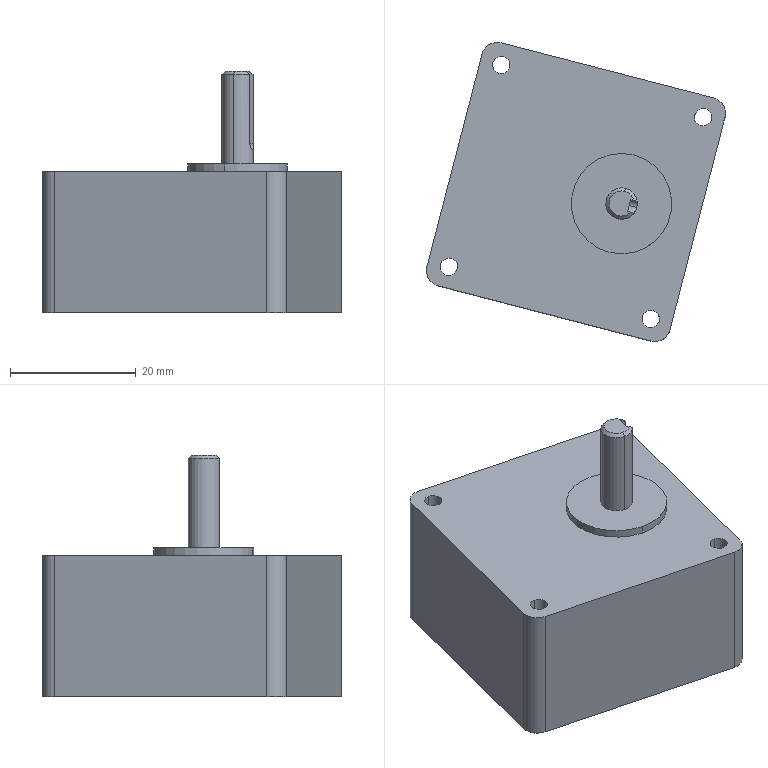Part | SolidWorks | features SplitBody 1 | 1 solid | 32 faces | box 47.65 x 47.65 x 38.5 mm | volume 35855 mm3 | cylinder 18 | plane 11 | cone 3 | commonest cylinder face diameters 2.75 x8 5 x6 2 x2 16 x2
STEP:
#1=CARTESIAN_POINT('',(-144.137,330.797,-440.116));
#2=VERTEX_POINT('',#1);
#3=CARTESIAN_POINT('',(-142.209,331.331,-440.116));
#4=VERTEX_POINT('',#3);
#5=CARTESIAN_POINT('',(-143.636,332.733,-440.116));
#6=DIRECTION('',(0.,0.,1.));
#7=DIRECTION('',(-0.2504,-0.9681,0.));
#8=AXIS2_PLACEMENT_3D('',#5,#6,#7);
#9=CIRCLE('',#8,2.);
#10=EDGE_CURVE('',#2,#4,#9,.T.);
#11=ORIENTED_EDGE('',*,*,#10,.F.);
#12=CARTESIAN_POINT('',(-144.262,330.313,-440.616));
#13=VERTEX_POINT('',#12);
#14=CARTESIAN_POINT('',(-144.137,330.797,-440.116));
#15=DIRECTION('',(-0.1771,-0.6846,-0.7071));
#16=VECTOR('',#15,1000.);
#17=LINE('',#14,#16);
#18=EDGE_CURVE('',#2,#13,#17,.T.);
#19=ORIENTED_EDGE('',*,*,#18,.T.);
#20=CARTESIAN_POINT('',(-141.668,331.191,-440.616));
#21=VERTEX_POINT('',#20);
#22=CARTESIAN_POINT('',(-143.636,332.733,-440.616));
#23=DIRECTION('',(0.,0.,-1.));
#24=DIRECTION('',(-0.2504,-0.9681,0.));
#25=AXIS2_PLACEMENT_3D('',#22,#23,#24);
#26=CIRCLE('',#25,2.5);
#27=EDGE_CURVE('',#21,#13,#26,.T.);
#28=ORIENTED_EDGE('',*,*,#27,.F.);
#29=CARTESIAN_POINT('',(-142.209,331.331,-440.116));
#30=CARTESIAN_POINT('',(-142.026,331.284,-440.279));
#31=CARTESIAN_POINT('',(-141.847,331.237,-440.447));
#32=CARTESIAN_POINT('',(-141.668,331.191,-440.616));
#33=B_SPLINE_CURVE_WITH_KNOTS('',3,(#29,#30,#31,#32),.UNSPECIFIED.,.F.,.F.,(4,4),(0.001662,0.002407),.UNSPECIFIED.);
#34=EDGE_CURVE('',#4,#21,#33,.T.);
#35=ORIENTED_EDGE('',*,*,#34,.F.);
#36=EDGE_LOOP('',(#11,#19,#28,#35));
#37=FACE_OUTER_BOUND('',#36,.T.);
#38=CARTESIAN_POINT('',(-143.636,332.733,-440.116));
#39=DIRECTION('',(0.,0.,-1.));
#40=DIRECTION('',(0.2504,0.9681,0.));
#41=AXIS2_PLACEMENT_3D('',#38,#39,#40);
#42=CONICAL_SURFACE('',#41,2.,0.7854);
#43=ADVANCED_FACE('',(#37),#42,.T.);
#44=ORIENTED_EDGE('',*,*,#18,.F.);
#45=CARTESIAN_POINT('',(-143.135,334.669,-440.116));
#46=VERTEX_POINT('',#45);
#47=CARTESIAN_POINT('',(-143.636,332.733,-440.116));
#48=DIRECTION('',(0.,0.,1.));
#49=DIRECTION('',(-0.2504,-0.9681,0.));
#50=AXIS2_PLACEMENT_3D('',#47,#48,#49);
#51=CIRCLE('',#50,2.);
#52=EDGE_CURVE('',#46,#2,#51,.T.);
#53=ORIENTED_EDGE('',*,*,#52,.F.);
#54=CARTESIAN_POINT('',(-143.01,335.153,-440.616));
#55=VERTEX_POINT('',#54);
#56=CARTESIAN_POINT('',(-143.135,334.669,-440.116));
#57=DIRECTION('',(0.1771,0.6846,-0.7071));
#58=VECTOR('',#57,1000.);
#59=LINE('',#56,#58);
#60=EDGE_CURVE('',#46,#55,#59,.T.);
#61=ORIENTED_EDGE('',*,*,#60,.T.);
#62=CARTESIAN_POINT('',(-143.636,332.733,-440.616));
#63=DIRECTION('',(0.,0.,-1.));
#64=DIRECTION('',(-0.2504,-0.9681,0.));
#65=AXIS2_PLACEMENT_3D('',#62,#63,#64);
#66=CIRCLE('',#65,2.5);
#67=EDGE_CURVE('',#13,#55,#66,.T.);
#68=ORIENTED_EDGE('',*,*,#67,.F.);
#69=EDGE_LOOP('',(#44,#53,#61,#68));
#70=FACE_OUTER_BOUND('',#69,.T.);
#71=CARTESIAN_POINT('',(-143.636,332.733,-440.116));
#72=DIRECTION('',(0.,0.,-1.));
#73=DIRECTION('',(0.2504,0.9681,0.));
#74=AXIS2_PLACEMENT_3D('',#71,#72,#73);
#75=CONICAL_SURFACE('',#74,2.,0.7854);
#76=ADVANCED_FACE('',(#70),#75,.T.);
#77=ORIENTED_EDGE('',*,*,#27,.T.);
#78=CARTESIAN_POINT('',(-144.262,330.313,-454.866));
#79=VERTEX_POINT('',#78);
#80=CARTESIAN_POINT('',(-144.262,330.313,-440.116));
#81=DIRECTION('',(0.,0.,-1.));
#82=VECTOR('',#81,1000.);
#83=LINE('',#80,#82);
#84=EDGE_CURVE('',#13,#79,#83,.T.);
#85=ORIENTED_EDGE('',*,*,#84,.T.);
#86=CARTESIAN_POINT('',(-143.01,335.153,-454.866));
#87=VERTEX_POINT('',#86);
#88=CARTESIAN_POINT('',(-143.636,332.733,-454.866));
#89=DIRECTION('',(0.,0.,-1.));
#90=DIRECTION('',(-0.2504,-0.9681,0.));
#91=AXIS2_PLACEMENT_3D('',#88,#89,#90);
#92=CIRCLE('',#91,2.5);
#93=EDGE_CURVE('',#87,#79,#92,.T.);
#94=ORIENTED_EDGE('',*,*,#93,.F.);
#95=CARTESIAN_POINT('',(-143.01,335.153,-440.116));
#96=DIRECTION('',(0.,0.,-1.));
#97=VECTOR('',#96,1000.);
#98=LINE('',#95,#97);
#99=EDGE_CURVE('',#55,#87,#98,.T.);
#100=ORIENTED_EDGE('',*,*,#99,.F.);
#101=CARTESIAN_POINT('',(-141.167,333.127,-440.616));
#102=VERTEX_POINT('',#101);
#103=CARTESIAN_POINT('',(-143.636,332.733,-440.616));
#104=DIRECTION('',(0.,0.,-1.));
#105=DIRECTION('',(-0.2504,-0.9681,0.));
#106=AXIS2_PLACEMENT_3D('',#103,#104,#105);
#107=CIRCLE('',#106,2.5);
#108=EDGE_CURVE('',#55,#102,#107,.T.);
#109=ORIENTED_EDGE('',*,*,#108,.T.);
#110=CARTESIAN_POINT('',(-141.167,333.127,-451.616));
#111=VERTEX_POINT('',#110);
#112=CARTESIAN_POINT('',(-141.167,333.127,-440.116));
#113=DIRECTION('',(0.,0.,-1.));
#114=VECTOR('',#113,1000.);
#115=LINE('',#112,#114);
#116=EDGE_CURVE('',#102,#111,#115,.T.);
#117=ORIENTED_EDGE('',*,*,#116,.T.);
#118=CARTESIAN_POINT('',(-141.216,332.107,-452.616));
#119=VERTEX_POINT('',#118);
#120=CARTESIAN_POINT('',(-141.167,333.127,-451.616));
#121=CARTESIAN_POINT('',(-141.167,333.127,-451.749));
#122=CARTESIAN_POINT('',(-141.162,333.098,-451.88));
#123=CARTESIAN_POINT('',(-141.149,332.991,-452.121));
#124=CARTESIAN_POINT('',(-141.141,332.912,-452.231));
#125=CARTESIAN_POINT('',(-141.134,332.722,-452.414));
#126=CARTESIAN_POINT('',(-141.136,332.609,-452.488));
#127=CARTESIAN_POINT('',(-141.16,332.367,-452.588));
#128=CARTESIAN_POINT('',(-141.182,332.236,-452.616));
#129=CARTESIAN_POINT('',(-141.216,332.107,-452.616));
#130=B_SPLINE_CURVE_WITH_KNOTS('',3,(#120,#121,#122,#123,#124,#125,#126,#127,#128,#129),.UNSPECIFIED.,.F.,.F.,(4,2,2,2,4),(0.,0.0003947,0.0007895,0.001184,0.001579),.UNSPECIFIED.);
#131=EDGE_CURVE('',#111,#119,#130,.T.);
#132=ORIENTED_EDGE('',*,*,#131,.T.);
#133=CARTESIAN_POINT('',(-141.668,331.191,-451.616));
#134=VERTEX_POINT('',#133);
#135=CARTESIAN_POINT('',(-141.216,332.107,-452.616));
#136=CARTESIAN_POINT('',(-141.249,331.978,-452.616));
#137=CARTESIAN_POINT('',(-141.292,331.854,-452.589));
#138=CARTESIAN_POINT('',(-141.389,331.629,-452.488));
#139=CARTESIAN_POINT('',(-141.443,331.529,-452.414));
#140=CARTESIAN_POINT('',(-141.54,331.366,-452.231));
#141=CARTESIAN_POINT('',(-141.586,331.301,-452.121));
#142=CARTESIAN_POINT('',(-141.649,331.214,-451.881));
#143=CARTESIAN_POINT('',(-141.668,331.191,-451.749));
#144=CARTESIAN_POINT('',(-141.668,331.191,-451.616));
#145=B_SPLINE_CURVE_WITH_KNOTS('',3,(#135,#136,#137,#138,#139,#140,#141,#142,#143,#144),.UNSPECIFIED.,.F.,.F.,(4,2,2,2,4),(0.,0.0003948,0.0007895,0.001184,0.001579),.UNSPECIFIED.);
#146=EDGE_CURVE('',#119,#134,#145,.T.);
#147=ORIENTED_EDGE('',*,*,#146,.T.);
#148=CARTESIAN_POINT('',(-141.668,331.191,-440.116));
#149=DIRECTION('',(0.,0.,1.));
#150=VECTOR('',#149,1000.);
#151=LINE('',#148,#150);
#152=EDGE_CURVE('',#134,#21,#151,.T.);
#153=ORIENTED_EDGE('',*,*,#152,.T.);
#154=EDGE_LOOP('',(#77,#85,#94,#100,#109,#117,#132,#147,#153));
#155=FACE_OUTER_BOUND('',#154,.T.);
#156=CARTESIAN_POINT('',(-143.636,332.733,-440.116));
#157=DIRECTION('',(0.,0.,-1.));
#158=DIRECTION('',(0.2504,0.9681,0.));
#159=AXIS2_PLACEMENT_3D('',#156,#157,#158);
#160=CYLINDRICAL_SURFACE('',#159,2.5);
#161=ADVANCED_FACE('',(#155),#160,.T.);
#162=CARTESIAN_POINT('',(-145.639,324.988,-454.866));
#163=VERTEX_POINT('',#162);
#164=CARTESIAN_POINT('',(-141.632,340.478,-454.866));
#165=VERTEX_POINT('',#164);
#166=CARTESIAN_POINT('',(-143.636,332.733,-454.866));
#167=DIRECTION('',(0.,0.,1.));
#168=DIRECTION('',(-0.2504,-0.9681,0.));
#169=AXIS2_PLACEMENT_3D('',#166,#167,#168);
#170=CIRCLE('',#169,8.);
#171=EDGE_CURVE('',#163,#165,#170,.T.);
#172=ORIENTED_EDGE('',*,*,#171,.F.);
#173=CARTESIAN_POINT('',(-145.639,324.988,-456.116));
#174=VERTEX_POINT('',#173);
#175=CARTESIAN_POINT('',(-145.639,324.988,-454.866));
#176=DIRECTION('',(0.,0.,-1.));
#177=VECTOR('',#176,1000.);
#178=LINE('',#175,#177);
#179=EDGE_CURVE('',#163,#174,#178,.T.);
#180=ORIENTED_EDGE('',*,*,#179,.T.);
#181=CARTESIAN_POINT('',(-141.632,340.478,-456.116));
#182=VERTEX_POINT('',#181);
#183=CARTESIAN_POINT('',(-143.636,332.733,-456.116));
#184=DIRECTION('',(0.,0.,1.));
#185=DIRECTION('',(-0.2504,-0.9681,0.));
#186=AXIS2_PLACEMENT_3D('',#183,#184,#185);
#187=CIRCLE('',#186,8.);
#188=EDGE_CURVE('',#174,#182,#187,.T.);
#189=ORIENTED_EDGE('',*,*,#188,.T.);
#190=CARTESIAN_POINT('',(-141.632,340.478,-454.866));
#191=DIRECTION('',(0.,0.,-1.));
#192=VECTOR('',#191,1000.);
#193=LINE('',#190,#192);
#194=EDGE_CURVE('',#165,#182,#193,.T.);
#195=ORIENTED_EDGE('',*,*,#194,.F.);
#196=EDGE_LOOP('',(#172,#180,#189,#195));
#197=FACE_OUTER_BOUND('',#196,.T.);
#198=CARTESIAN_POINT('',(-143.636,332.733,-454.866));
#199=DIRECTION('',(0.,0.,-1.));
#200=DIRECTION('',(0.2504,0.9681,0.));
#201=AXIS2_PLACEMENT_3D('',#198,#199,#200);
#202=CYLINDRICAL_SURFACE('',#201,8.);
#203=ADVANCED_FACE('',(#197),#202,.T.);
#204=CARTESIAN_POINT('',(-138.627,315.693,-456.116));
#205=VERTEX_POINT('',#204);
#206=CARTESIAN_POINT('',(-139.315,313.031,-456.116));
#207=VERTEX_POINT('',#206);
#208=CARTESIAN_POINT('',(-138.971,314.362,-456.116));
#209=DIRECTION('',(0.,0.,1.));
#210=DIRECTION('',(-0.2504,-0.9681,0.));
#211=AXIS2_PLACEMENT_3D('',#208,#209,#210);
#212=CIRCLE('',#211,1.375);
#213=EDGE_CURVE('',#205,#207,#212,.T.);
#214=ORIENTED_EDGE('',*,*,#213,.T.);
#215=CARTESIAN_POINT('',(-139.315,313.031,-478.616));
#216=VERTEX_POINT('',#215);
#217=CARTESIAN_POINT('',(-139.315,313.031,-456.116));
#218=DIRECTION('',(0.,0.,-1.));
#219=VECTOR('',#218,1000.);
#220=LINE('',#217,#219);
#221=EDGE_CURVE('',#207,#216,#220,.T.);
#222=ORIENTED_EDGE('',*,*,#221,.T.);
#223=CARTESIAN_POINT('',(-138.627,315.693,-478.616));
#224=VERTEX_POINT('',#223);
#225=CARTESIAN_POINT('',(-138.971,314.362,-478.616));
#226=DIRECTION('',(0.,0.,1.));
#227=DIRECTION('',(-0.2504,-0.9681,0.));
#228=AXIS2_PLACEMENT_3D('',#225,#226,#227);
#229=CIRCLE('',#228,1.375);
#230=EDGE_CURVE('',#224,#216,#229,.T.);
#231=ORIENTED_EDGE('',*,*,#230,.F.);
#232=CARTESIAN_POINT('',(-138.627,315.693,-456.116));
#233=DIRECTION('',(0.,0.,-1.));
#234=VECTOR('',#233,1000.);
#235=LINE('',#232,#234);
#236=EDGE_CURVE('',#205,#224,#235,.T.);
#237=ORIENTED_EDGE('',*,*,#236,.F.);
#238=EDGE_LOOP('',(#214,#222,#231,#237));
#239=FACE_OUTER_BOUND('',#238,.T.);
#240=CARTESIAN_POINT('',(-138.971,314.362,-456.116));
#241=DIRECTION('',(0.,0.,-1.));
#242=DIRECTION('',(0.2504,0.9681,0.));
#243=AXIS2_PLACEMENT_3D('',#240,#241,#242);
#244=CYLINDRICAL_SURFACE('',#243,1.375);
#245=ADVANCED_FACE('',(#239),#244,.F.);
#246=CARTESIAN_POINT('',(-170.802,324.017,-456.116));
#247=VERTEX_POINT('',#246);
#248=CARTESIAN_POINT('',(-171.49,321.354,-456.116));
#249=VERTEX_POINT('',#248);
#250=CARTESIAN_POINT('',(-171.146,322.685,-456.116));
#251=DIRECTION('',(0.,0.,1.));
#252=DIRECTION('',(-0.2504,-0.9681,0.));
#253=AXIS2_PLACEMENT_3D('',#250,#251,#252);
#254=CIRCLE('',#253,1.375);
#255=EDGE_CURVE('',#247,#249,#254,.T.);
#256=ORIENTED_EDGE('',*,*,#255,.T.);
#257=CARTESIAN_POINT('',(-171.49,321.354,-478.616));
#258=VERTEX_POINT('',#257);
#259=CARTESIAN_POINT('',(-171.49,321.354,-456.116));
#260=DIRECTION('',(0.,0.,-1.));
#261=VECTOR('',#260,1000.);
#262=LINE('',#259,#261);
#263=EDGE_CURVE('',#249,#258,#262,.T.);
#264=ORIENTED_EDGE('',*,*,#263,.T.);
#265=CARTESIAN_POINT('',(-170.802,324.017,-478.616));
#266=VERTEX_POINT('',#265);
#267=CARTESIAN_POINT('',(-171.146,322.685,-478.616));
#268=DIRECTION('',(0.,0.,1.));
#269=DIRECTION('',(-0.2504,-0.9681,0.));
#270=AXIS2_PLACEMENT_3D('',#267,#268,#269);
#271=CIRCLE('',#270,1.375);
#272=EDGE_CURVE('',#266,#258,#271,.T.);
#273=ORIENTED_EDGE('',*,*,#272,.F.);
#274=CARTESIAN_POINT('',(-170.802,324.017,-456.116));
#275=DIRECTION('',(0.,0.,-1.));
#276=VECTOR('',#275,1000.);
#277=LINE('',#274,#276);
#278=EDGE_CURVE('',#247,#266,#277,.T.);
#279=ORIENTED_EDGE('',*,*,#278,.F.);
#280=EDGE_LOOP('',(#256,#264,#273,#279));
#281=FACE_OUTER_BOUND('',#280,.T.);
#282=CARTESIAN_POINT('',(-171.146,322.685,-456.116));
#283=DIRECTION('',(0.,0.,-1.));
#284=DIRECTION('',(0.2504,0.9681,0.));
#285=AXIS2_PLACEMENT_3D('',#282,#283,#284);
#286=CYLINDRICAL_SURFACE('',#285,1.375);
#287=ADVANCED_FACE('',(#281),#286,.F.);
#288=CARTESIAN_POINT('',(-162.478,356.191,-456.116));
#289=VERTEX_POINT('',#288);
#290=CARTESIAN_POINT('',(-163.167,353.529,-456.116));
#291=VERTEX_POINT('',#290);
#292=CARTESIAN_POINT('',(-162.823,354.86,-456.116));
#293=DIRECTION('',(0.,0.,1.));
#294=DIRECTION('',(-0.2504,-0.9681,0.));
#295=AXIS2_PLACEMENT_3D('',#292,#293,#294);
#296=CIRCLE('',#295,1.375);
#297=EDGE_CURVE('',#289,#291,#296,.T.);
#298=ORIENTED_EDGE('',*,*,#297,.T.);
#299=CARTESIAN_POINT('',(-163.167,353.529,-478.616));
#300=VERTEX_POINT('',#299);
#301=CARTESIAN_POINT('',(-163.167,353.529,-456.116));
#302=DIRECTION('',(0.,0.,-1.));
#303=VECTOR('',#302,1000.);
#304=LINE('',#301,#303);
#305=EDGE_CURVE('',#291,#300,#304,.T.);
#306=ORIENTED_EDGE('',*,*,#305,.T.);
#307=CARTESIAN_POINT('',(-162.478,356.191,-478.616));
#308=VERTEX_POINT('',#307);
#309=CARTESIAN_POINT('',(-162.823,354.86,-478.616));
#310=DIRECTION('',(0.,0.,1.));
#311=DIRECTION('',(-0.2504,-0.9681,0.));
#312=AXIS2_PLACEMENT_3D('',#309,#310,#311);
#313=CIRCLE('',#312,1.375);
#314=EDGE_CURVE('',#308,#300,#313,.T.);
#315=ORIENTED_EDGE('',*,*,#314,.F.);
#316=CARTESIAN_POINT('',(-162.478,356.191,-456.116));
#317=DIRECTION('',(0.,0.,-1.));
#318=VECTOR('',#317,1000.);
#319=LINE('',#316,#318);
#320=EDGE_CURVE('',#289,#308,#319,.T.);
#321=ORIENTED_EDGE('',*,*,#320,.F.);
#322=EDGE_LOOP('',(#298,#306,#315,#321));
#323=FACE_OUTER_BOUND('',#322,.T.);
#324=CARTESIAN_POINT('',(-162.823,354.86,-456.116));
#325=DIRECTION('',(0.,0.,-1.));
#326=DIRECTION('',(0.2504,0.9681,0.));
#327=AXIS2_PLACEMENT_3D('',#324,#325,#326);
#328=CYLINDRICAL_SURFACE('',#327,1.375);
#329=ADVANCED_FACE('',(#323),#328,.F.);
#330=CARTESIAN_POINT('',(-130.304,347.868,-456.116));
#331=VERTEX_POINT('',#330);
#332=CARTESIAN_POINT('',(-130.992,345.206,-456.116));
#333=VERTEX_POINT('',#332);
#334=CARTESIAN_POINT('',(-130.648,346.537,-456.116));
#335=DIRECTION('',(0.,0.,1.));
#336=DIRECTION('',(-0.2504,-0.9681,0.));
#337=AXIS2_PLACEMENT_3D('',#334,#335,#336);
#338=CIRCLE('',#337,1.375);
#339=EDGE_CURVE('',#331,#333,#338,.T.);
#340=ORIENTED_EDGE('',*,*,#339,.T.);
#341=CARTESIAN_POINT('',(-130.992,345.206,-478.616));
#342=VERTEX_POINT('',#341);
#343=CARTESIAN_POINT('',(-130.992,345.206,-456.116));
#344=DIRECTION('',(0.,0.,-1.));
#345=VECTOR('',#344,1000.);
#346=LINE('',#343,#345);
#347=EDGE_CURVE('',#333,#342,#346,.T.);
#348=ORIENTED_EDGE('',*,*,#347,.T.);
#349=CARTESIAN_POINT('',(-130.304,347.868,-478.616));
#350=VERTEX_POINT('',#349);
#351=CARTESIAN_POINT('',(-130.648,346.537,-478.616));
#352=DIRECTION('',(0.,0.,1.));
#353=DIRECTION('',(-0.2504,-0.9681,0.));
#354=AXIS2_PLACEMENT_3D('',#351,#352,#353);
#355=CIRCLE('',#354,1.375);
#356=EDGE_CURVE('',#350,#342,#355,.T.);
#357=ORIENTED_EDGE('',*,*,#356,.F.);
#358=CARTESIAN_POINT('',(-130.304,347.868,-456.116));
#359=DIRECTION('',(0.,0.,-1.));
#360=VECTOR('',#359,1000.);
#361=LINE('',#358,#360);
#362=EDGE_CURVE('',#331,#350,#361,.T.);
#363=ORIENTED_EDGE('',*,*,#362,.F.);
#364=EDGE_LOOP('',(#340,#348,#357,#363));
#365=FACE_OUTER_BOUND('',#364,.T.);
#366=CARTESIAN_POINT('',(-130.648,346.537,-456.116));
#367=DIRECTION('',(0.,0.,-1.));
#368=DIRECTION('',(0.2504,0.9681,0.));
#369=AXIS2_PLACEMENT_3D('',#366,#367,#368);
#370=CYLINDRICAL_SURFACE('',#369,1.375);
#371=ADVANCED_FACE('',(#365),#370,.F.);
#372=CARTESIAN_POINT('',(-143.636,332.733,-454.866));
#373=DIRECTION('',(0.,0.,1.));
#374=DIRECTION('',(-0.2504,-0.9681,0.));
#375=AXIS2_PLACEMENT_3D('',#372,#373,#374);
#376=CIRCLE('',#375,8.);
#377=EDGE_CURVE('',#165,#163,#376,.T.);
#378=ORIENTED_EDGE('',*,*,#377,.T.);
#379=ORIENTED_EDGE('',*,*,#171,.T.);
#380=EDGE_LOOP('',(#378,#379));
#381=FACE_OUTER_BOUND('',#380,.T.);
#382=ORIENTED_EDGE('',*,*,#93,.T.);
#383=CARTESIAN_POINT('',(-143.636,332.733,-454.866));
#384=DIRECTION('',(0.,0.,-1.));
#385=DIRECTION('',(-0.2504,-0.9681,0.));
#386=AXIS2_PLACEMENT_3D('',#383,#384,#385);
#387=CIRCLE('',#386,2.5);
#388=EDGE_CURVE('',#79,#87,#387,.T.);
#389=ORIENTED_EDGE('',*,*,#388,.T.);
#390=EDGE_LOOP('',(#382,#389));
#391=FACE_BOUND('',#390,.T.);
#392=CARTESIAN_POINT('',(-143.636,332.733,-454.866));
#393=DIRECTION('',(0.,0.,1.));
#394=DIRECTION('',(-0.2504,-0.9681,0.));
#395=AXIS2_PLACEMENT_3D('',#392,#393,#394);
#396=PLANE('',#395);
#397=ADVANCED_FACE('',(#381,#391),#396,.T.);
#398=ORIENTED_EDGE('',*,*,#213,.F.);
#399=CARTESIAN_POINT('',(-138.971,314.362,-456.116));
#400=DIRECTION('',(0.,0.,1.));
#401=DIRECTION('',(-0.2504,-0.9681,0.));
#402=AXIS2_PLACEMENT_3D('',#399,#400,#401);
#403=CIRCLE('',#402,1.375);
#404=EDGE_CURVE('',#207,#205,#403,.T.);
#405=ORIENTED_EDGE('',*,*,#404,.F.);
#406=EDGE_LOOP('',(#398,#405));
#407=FACE_BOUND('',#406,.T.);
#408=ORIENTED_EDGE('',*,*,#297,.F.);
#409=CARTESIAN_POINT('',(-162.823,354.86,-456.116));
#410=DIRECTION('',(0.,0.,1.));
#411=DIRECTION('',(-0.2504,-0.9681,0.));
#412=AXIS2_PLACEMENT_3D('',#409,#410,#411);
#413=CIRCLE('',#412,1.375);
#414=EDGE_CURVE('',#291,#289,#413,.T.);
#415=ORIENTED_EDGE('',*,*,#414,.F.);
#416=EDGE_LOOP('',(#408,#415));
#417=FACE_BOUND('',#416,.T.);
#418=CARTESIAN_POINT('',(-162.83,358.357,-456.116));
#419=VERTEX_POINT('',#418);
#420=CARTESIAN_POINT('',(-165.877,356.562,-456.116));
#421=VERTEX_POINT('',#420);
#422=CARTESIAN_POINT('',(-163.457,355.936,-456.116));
#423=DIRECTION('',(0.,0.,1.));
#424=DIRECTION('',(-0.2504,-0.9681,0.));
#425=AXIS2_PLACEMENT_3D('',#422,#423,#424);
#426=CIRCLE('',#425,2.5);
#427=EDGE_CURVE('',#419,#421,#426,.T.);
#428=ORIENTED_EDGE('',*,*,#427,.T.);
#429=CARTESIAN_POINT('',(-174.642,322.678,-456.116));
#430=VERTEX_POINT('',#429);
#431=CARTESIAN_POINT('',(-165.877,356.562,-456.116));
#432=DIRECTION('',(-0.2504,-0.9681,0.));
#433=VECTOR('',#432,1000.);
#434=LINE('',#431,#433);
#435=EDGE_CURVE('',#421,#430,#434,.T.);
#436=ORIENTED_EDGE('',*,*,#435,.T.);
#437=CARTESIAN_POINT('',(-172.848,319.631,-456.116));
#438=VERTEX_POINT('',#437);
#439=CARTESIAN_POINT('',(-172.222,322.052,-456.116));
#440=DIRECTION('',(0.,0.,1.));
#441=DIRECTION('',(-0.2504,-0.9681,0.));
#442=AXIS2_PLACEMENT_3D('',#439,#440,#441);
#443=CIRCLE('',#442,2.5);
#444=EDGE_CURVE('',#430,#438,#443,.T.);
#445=ORIENTED_EDGE('',*,*,#444,.T.);
#446=CARTESIAN_POINT('',(-138.963,310.866,-456.116));
#447=VERTEX_POINT('',#446);
#448=CARTESIAN_POINT('',(-172.848,319.631,-456.116));
#449=DIRECTION('',(0.9681,-0.2504,0.));
#450=VECTOR('',#449,1000.);
#451=LINE('',#448,#450);
#452=EDGE_CURVE('',#438,#447,#451,.T.);
#453=ORIENTED_EDGE('',*,*,#452,.T.);
#454=CARTESIAN_POINT('',(-135.917,312.66,-456.116));
#455=VERTEX_POINT('',#454);
#456=CARTESIAN_POINT('',(-138.337,313.286,-456.116));
#457=DIRECTION('',(0.,0.,1.));
#458=DIRECTION('',(-0.2504,-0.9681,0.));
#459=AXIS2_PLACEMENT_3D('',#456,#457,#458);
#460=CIRCLE('',#459,2.5);
#461=EDGE_CURVE('',#447,#455,#460,.T.);
#462=ORIENTED_EDGE('',*,*,#461,.T.);
#463=CARTESIAN_POINT('',(-127.152,346.545,-456.116));
#464=VERTEX_POINT('',#463);
#465=CARTESIAN_POINT('',(-135.917,312.66,-456.116));
#466=DIRECTION('',(0.2504,0.9681,0.));
#467=VECTOR('',#466,1000.);
#468=LINE('',#465,#467);
#469=EDGE_CURVE('',#455,#464,#468,.T.);
#470=ORIENTED_EDGE('',*,*,#469,.T.);
#471=CARTESIAN_POINT('',(-128.946,349.591,-456.116));
#472=VERTEX_POINT('',#471);
#473=CARTESIAN_POINT('',(-129.572,347.171,-456.116));
#474=DIRECTION('',(0.,0.,1.));
#475=DIRECTION('',(-0.2504,-0.9681,0.));
#476=AXIS2_PLACEMENT_3D('',#473,#474,#475);
#477=CIRCLE('',#476,2.5);
#478=EDGE_CURVE('',#464,#472,#477,.T.);
#479=ORIENTED_EDGE('',*,*,#478,.T.);
#480=CARTESIAN_POINT('',(-128.946,349.591,-456.116));
#481=DIRECTION('',(-0.9681,0.2504,0.));
#482=VECTOR('',#481,1000.);
#483=LINE('',#480,#482);
#484=EDGE_CURVE('',#472,#419,#483,.T.);
#485=ORIENTED_EDGE('',*,*,#484,.T.);
#486=EDGE_LOOP('',(#428,#436,#445,#453,#462,#470,#479,#485));
#487=FACE_OUTER_BOUND('',#486,.T.);
#488=ORIENTED_EDGE('',*,*,#339,.F.);
#489=CARTESIAN_POINT('',(-130.648,346.537,-456.116));
#490=DIRECTION('',(0.,0.,1.));
#491=DIRECTION('',(-0.2504,-0.9681,0.));
#492=AXIS2_PLACEMENT_3D('',#489,#490,#491);
#493=CIRCLE('',#492,1.375);
#494=EDGE_CURVE('',#333,#331,#493,.T.);
#495=ORIENTED_EDGE('',*,*,#494,.F.);
#496=EDGE_LOOP('',(#488,#495));
#497=FACE_BOUND('',#496,.T.);
#498=ORIENTED_EDGE('',*,*,#255,.F.);
#499=CARTESIAN_POINT('',(-171.146,322.685,-456.116));
#500=DIRECTION('',(0.,0.,1.));
#501=DIRECTION('',(-0.2504,-0.9681,0.));
#502=AXIS2_PLACEMENT_3D('',#499,#500,#501);
#503=CIRCLE('',#502,1.375);
#504=EDGE_CURVE('',#249,#247,#503,.T.);
#505=ORIENTED_EDGE('',*,*,#504,.F.);
#506=EDGE_LOOP('',(#498,#505));
#507=FACE_BOUND('',#506,.T.);
#508=CARTESIAN_POINT('',(-143.636,332.733,-456.116));
#509=DIRECTION('',(0.,0.,1.));
#510=DIRECTION('',(-0.2504,-0.9681,0.));
#511=AXIS2_PLACEMENT_3D('',#508,#509,#510);
#512=CIRCLE('',#511,8.);
#513=EDGE_CURVE('',#182,#174,#512,.T.);
#514=ORIENTED_EDGE('',*,*,#513,.F.);
#515=ORIENTED_EDGE('',*,*,#188,.F.);
#516=EDGE_LOOP('',(#514,#515));
#517=FACE_BOUND('',#516,.T.);
#518=CARTESIAN_POINT('',(-163.457,355.936,-456.116));
#519=DIRECTION('',(0.,0.,1.));
#520=DIRECTION('',(-0.2504,-0.9681,0.));
#521=AXIS2_PLACEMENT_3D('',#518,#519,#520);
#522=PLANE('',#521);
#523=ADVANCED_FACE('',(#407,#417,#487,#497,#507,#517),#522,.T.);
#524=ORIENTED_EDGE('',*,*,#272,.T.);
#525=CARTESIAN_POINT('',(-171.146,322.685,-478.616));
#526=DIRECTION('',(0.,0.,1.));
#527=DIRECTION('',(-0.2504,-0.9681,0.));
#528=AXIS2_PLACEMENT_3D('',#525,#526,#527);
#529=CIRCLE('',#528,1.375);
#530=EDGE_CURVE('',#258,#266,#529,.T.);
#531=ORIENTED_EDGE('',*,*,#530,.T.);
#532=EDGE_LOOP('',(#524,#531));
#533=FACE_BOUND('',#532,.T.);
#534=ORIENTED_EDGE('',*,*,#356,.T.);
#535=CARTESIAN_POINT('',(-130.648,346.537,-478.616));
#536=DIRECTION('',(0.,0.,1.));
#537=DIRECTION('',(-0.2504,-0.9681,0.));
#538=AXIS2_PLACEMENT_3D('',#535,#536,#537);
#539=CIRCLE('',#538,1.375);
#540=EDGE_CURVE('',#342,#350,#539,.T.);
#541=ORIENTED_EDGE('',*,*,#540,.T.);
#542=EDGE_LOOP('',(#534,#541));
#543=FACE_BOUND('',#542,.T.);
#544=CARTESIAN_POINT('',(-162.83,358.357,-478.616));
#545=VERTEX_POINT('',#544);
#546=CARTESIAN_POINT('',(-165.877,356.562,-478.616));
#547=VERTEX_POINT('',#546);
#548=CARTESIAN_POINT('',(-163.457,355.936,-478.616));
#549=DIRECTION('',(0.,0.,1.));
#550=DIRECTION('',(-0.2504,-0.9681,0.));
#551=AXIS2_PLACEMENT_3D('',#548,#549,#550);
#552=CIRCLE('',#551,2.5);
#553=EDGE_CURVE('',#545,#547,#552,.T.);
#554=ORIENTED_EDGE('',*,*,#553,.F.);
#555=CARTESIAN_POINT('',(-128.946,349.591,-478.616));
#556=VERTEX_POINT('',#555);
#557=CARTESIAN_POINT('',(-128.946,349.591,-478.616));
#558=DIRECTION('',(-0.9681,0.2504,0.));
#559=VECTOR('',#558,1000.);
#560=LINE('',#557,#559);
#561=EDGE_CURVE('',#556,#545,#560,.T.);
#562=ORIENTED_EDGE('',*,*,#561,.F.);
#563=CARTESIAN_POINT('',(-127.152,346.545,-478.616));
#564=VERTEX_POINT('',#563);
#565=CARTESIAN_POINT('',(-129.572,347.171,-478.616));
#566=DIRECTION('',(0.,0.,1.));
#567=DIRECTION('',(-0.2504,-0.9681,0.));
#568=AXIS2_PLACEMENT_3D('',#565,#566,#567);
#569=CIRCLE('',#568,2.5);
#570=EDGE_CURVE('',#564,#556,#569,.T.);
#571=ORIENTED_EDGE('',*,*,#570,.F.);
#572=CARTESIAN_POINT('',(-135.917,312.66,-478.616));
#573=VERTEX_POINT('',#572);
#574=CARTESIAN_POINT('',(-135.917,312.66,-478.616));
#575=DIRECTION('',(0.2504,0.9681,0.));
#576=VECTOR('',#575,1000.);
#577=LINE('',#574,#576);
#578=EDGE_CURVE('',#573,#564,#577,.T.);
#579=ORIENTED_EDGE('',*,*,#578,.F.);
#580=CARTESIAN_POINT('',(-138.963,310.866,-478.616));
#581=VERTEX_POINT('',#580);
#582=CARTESIAN_POINT('',(-138.337,313.286,-478.616));
#583=DIRECTION('',(0.,0.,1.));
#584=DIRECTION('',(-0.2504,-0.9681,0.));
#585=AXIS2_PLACEMENT_3D('',#582,#583,#584);
#586=CIRCLE('',#585,2.5);
#587=EDGE_CURVE('',#581,#573,#586,.T.);
#588=ORIENTED_EDGE('',*,*,#587,.F.);
#589=CARTESIAN_POINT('',(-172.848,319.631,-478.616));
#590=VERTEX_POINT('',#589);
#591=CARTESIAN_POINT('',(-172.848,319.631,-478.616));
#592=DIRECTION('',(0.9681,-0.2504,0.));
#593=VECTOR('',#592,1000.);
#594=LINE('',#591,#593);
#595=EDGE_CURVE('',#590,#581,#594,.T.);
#596=ORIENTED_EDGE('',*,*,#595,.F.);
#597=CARTESIAN_POINT('',(-174.642,322.678,-478.616));
#598=VERTEX_POINT('',#597);
#599=CARTESIAN_POINT('',(-172.222,322.052,-478.616));
#600=DIRECTION('',(0.,0.,1.));
#601=DIRECTION('',(-0.2504,-0.9681,0.));
#602=AXIS2_PLACEMENT_3D('',#599,#600,#601);
#603=CIRCLE('',#602,2.5);
#604=EDGE_CURVE('',#598,#590,#603,.T.);
#605=ORIENTED_EDGE('',*,*,#604,.F.);
#606=CARTESIAN_POINT('',(-165.877,356.562,-478.616));
#607=DIRECTION('',(-0.2504,-0.9681,0.));
#608=VECTOR('',#607,1000.);
#609=LINE('',#606,#608);
#610=EDGE_CURVE('',#547,#598,#609,.T.);
#611=ORIENTED_EDGE('',*,*,#610,.F.);
#612=EDGE_LOOP('',(#554,#562,#571,#579,#588,#596,#605,#611));
#613=FACE_OUTER_BOUND('',#612,.T.);
#614=ORIENTED_EDGE('',*,*,#314,.T.);
#615=CARTESIAN_POINT('',(-162.823,354.86,-478.616));
#616=DIRECTION('',(0.,0.,1.));
#617=DIRECTION('',(-0.2504,-0.9681,0.));
#618=AXIS2_PLACEMENT_3D('',#615,#616,#617);
#619=CIRCLE('',#618,1.375);
#620=EDGE_CURVE('',#300,#308,#619,.T.);
#621=ORIENTED_EDGE('',*,*,#620,.T.);
#622=EDGE_LOOP('',(#614,#621));
#623=FACE_BOUND('',#622,.T.);
#624=ORIENTED_EDGE('',*,*,#230,.T.);
#625=CARTESIAN_POINT('',(-138.971,314.362,-478.616));
#626=DIRECTION('',(0.,0.,1.));
#627=DIRECTION('',(-0.2504,-0.9681,0.));
#628=AXIS2_PLACEMENT_3D('',#625,#626,#627);
#629=CIRCLE('',#628,1.375);
#630=EDGE_CURVE('',#216,#224,#629,.T.);
#631=ORIENTED_EDGE('',*,*,#630,.T.);
#632=EDGE_LOOP('',(#624,#631));
#633=FACE_BOUND('',#632,.T.);
#634=CARTESIAN_POINT('',(-163.457,355.936,-478.616));
#635=DIRECTION('',(0.,0.,1.));
#636=DIRECTION('',(-0.2504,-0.9681,0.));
#637=AXIS2_PLACEMENT_3D('',#634,#635,#636);
#638=PLANE('',#637);
#639=ADVANCED_FACE('',(#533,#543,#613,#623,#633),#638,.F.);
#640=ORIENTED_EDGE('',*,*,#553,.T.);
#641=CARTESIAN_POINT('',(-165.877,356.562,-456.116));
#642=DIRECTION('',(0.,0.,-1.));
#643=VECTOR('',#642,1000.);
#644=LINE('',#641,#643);
#645=EDGE_CURVE('',#421,#547,#644,.T.);
#646=ORIENTED_EDGE('',*,*,#645,.F.);
#647=ORIENTED_EDGE('',*,*,#427,.F.);
#648=CARTESIAN_POINT('',(-162.83,358.357,-456.116));
#649=DIRECTION('',(0.,0.,-1.));
#650=VECTOR('',#649,1000.);
#651=LINE('',#648,#650);
#652=EDGE_CURVE('',#419,#545,#651,.T.);
#653=ORIENTED_EDGE('',*,*,#652,.T.);
#654=EDGE_LOOP('',(#640,#646,#647,#653));
#655=FACE_OUTER_BOUND('',#654,.T.);
#656=CARTESIAN_POINT('',(-163.457,355.936,-456.116));
#657=DIRECTION('',(0.,0.,-1.));
#658=DIRECTION('',(0.2504,0.9681,0.));
#659=AXIS2_PLACEMENT_3D('',#656,#657,#658);
#660=CYLINDRICAL_SURFACE('',#659,2.5);
#661=ADVANCED_FACE('',(#655),#660,.T.);
#662=ORIENTED_EDGE('',*,*,#610,.T.);
#663=CARTESIAN_POINT('',(-174.642,322.678,-456.116));
#664=DIRECTION('',(0.,0.,-1.));
#665=VECTOR('',#664,1000.);
#666=LINE('',#663,#665);
#667=EDGE_CURVE('',#430,#598,#666,.T.);
#668=ORIENTED_EDGE('',*,*,#667,.F.);
#669=ORIENTED_EDGE('',*,*,#435,.F.);
#670=ORIENTED_EDGE('',*,*,#645,.T.);
#671=EDGE_LOOP('',(#662,#668,#669,#670));
#672=FACE_OUTER_BOUND('',#671,.T.);
#673=CARTESIAN_POINT('',(-165.877,356.562,-456.116));
#674=DIRECTION('',(0.9681,-0.2504,0.));
#675=DIRECTION('',(0.,0.,1.));
#676=AXIS2_PLACEMENT_3D('',#673,#674,#675);
#677=PLANE('',#676);
#678=ADVANCED_FACE('',(#672),#677,.F.);
#679=ORIENTED_EDGE('',*,*,#604,.T.);
#680=CARTESIAN_POINT('',(-172.848,319.631,-456.116));
#681=DIRECTION('',(0.,0.,-1.));
#682=VECTOR('',#681,1000.);
#683=LINE('',#680,#682);
#684=EDGE_CURVE('',#438,#590,#683,.T.);
#685=ORIENTED_EDGE('',*,*,#684,.F.);
#686=ORIENTED_EDGE('',*,*,#444,.F.);
#687=ORIENTED_EDGE('',*,*,#667,.T.);
#688=EDGE_LOOP('',(#679,#685,#686,#687));
#689=FACE_OUTER_BOUND('',#688,.T.);
#690=CARTESIAN_POINT('',(-172.222,322.052,-456.116));
#691=DIRECTION('',(0.,0.,-1.));
#692=DIRECTION('',(0.2504,0.9681,0.));
#693=AXIS2_PLACEMENT_3D('',#690,#691,#692);
#694=CYLINDRICAL_SURFACE('',#693,2.5);
#695=ADVANCED_FACE('',(#689),#694,.T.);
#696=ORIENTED_EDGE('',*,*,#595,.T.);
#697=CARTESIAN_POINT('',(-138.963,310.866,-456.116));
#698=DIRECTION('',(0.,0.,-1.));
#699=VECTOR('',#698,1000.);
#700=LINE('',#697,#699);
#701=EDGE_CURVE('',#447,#581,#700,.T.);
#702=ORIENTED_EDGE('',*,*,#701,.F.);
#703=ORIENTED_EDGE('',*,*,#452,.F.);
#704=ORIENTED_EDGE('',*,*,#684,.T.);
#705=EDGE_LOOP('',(#696,#702,#703,#704));
#706=FACE_OUTER_BOUND('',#705,.T.);
#707=CARTESIAN_POINT('',(-172.848,319.631,-456.116));
#708=DIRECTION('',(0.2504,0.9681,0.));
#709=DIRECTION('',(-0.9681,0.2504,0.));
#710=AXIS2_PLACEMENT_3D('',#707,#708,#709);
#711=PLANE('',#710);
#712=ADVANCED_FACE('',(#706),#711,.F.);
#713=ORIENTED_EDGE('',*,*,#587,.T.);
#714=CARTESIAN_POINT('',(-135.917,312.66,-456.116));
#715=DIRECTION('',(0.,0.,-1.));
#716=VECTOR('',#715,1000.);
#717=LINE('',#714,#716);
#718=EDGE_CURVE('',#455,#573,#717,.T.);
#719=ORIENTED_EDGE('',*,*,#718,.F.);
#720=ORIENTED_EDGE('',*,*,#461,.F.);
#721=ORIENTED_EDGE('',*,*,#701,.T.);
#722=EDGE_LOOP('',(#713,#719,#720,#721));
#723=FACE_OUTER_BOUND('',#722,.T.);
#724=CARTESIAN_POINT('',(-138.337,313.286,-456.116));
#725=DIRECTION('',(0.,0.,-1.));
#726=DIRECTION('',(0.2504,0.9681,0.));
#727=AXIS2_PLACEMENT_3D('',#724,#725,#726);
#728=CYLINDRICAL_SURFACE('',#727,2.5);
#729=ADVANCED_FACE('',(#723),#728,.T.);
#730=ORIENTED_EDGE('',*,*,#578,.T.);
#731=CARTESIAN_POINT('',(-127.152,346.545,-456.116));
#732=DIRECTION('',(0.,0.,-1.));
#733=VECTOR('',#732,1000.);
#734=LINE('',#731,#733);
#735=EDGE_CURVE('',#464,#564,#734,.T.);
#736=ORIENTED_EDGE('',*,*,#735,.F.);
#737=ORIENTED_EDGE('',*,*,#469,.F.);
#738=ORIENTED_EDGE('',*,*,#718,.T.);
#739=EDGE_LOOP('',(#730,#736,#737,#738));
#740=FACE_OUTER_BOUND('',#739,.T.);
#741=CARTESIAN_POINT('',(-135.917,312.66,-456.116));
#742=DIRECTION('',(-0.9681,0.2504,0.));
#743=DIRECTION('',(0.,0.,-1.));
#744=AXIS2_PLACEMENT_3D('',#741,#742,#743);
#745=PLANE('',#744);
#746=ADVANCED_FACE('',(#740),#745,.F.);
#747=ORIENTED_EDGE('',*,*,#570,.T.);
#748=CARTESIAN_POINT('',(-128.946,349.591,-456.116));
#749=DIRECTION('',(0.,0.,-1.));
#750=VECTOR('',#749,1000.);
#751=LINE('',#748,#750);
#752=EDGE_CURVE('',#472,#556,#751,.T.);
#753=ORIENTED_EDGE('',*,*,#752,.F.);
#754=ORIENTED_EDGE('',*,*,#478,.F.);
#755=ORIENTED_EDGE('',*,*,#735,.T.);
#756=EDGE_LOOP('',(#747,#753,#754,#755));
#757=FACE_OUTER_BOUND('',#756,.T.);
#758=CARTESIAN_POINT('',(-129.572,347.171,-456.116));
#759=DIRECTION('',(0.,0.,-1.));
#760=DIRECTION('',(0.2504,0.9681,0.));
#761=AXIS2_PLACEMENT_3D('',#758,#759,#760);
#762=CYLINDRICAL_SURFACE('',#761,2.5);
#763=ADVANCED_FACE('',(#757),#762,.T.);
#764=ORIENTED_EDGE('',*,*,#561,.T.);
#765=ORIENTED_EDGE('',*,*,#652,.F.);
#766=ORIENTED_EDGE('',*,*,#484,.F.);
#767=ORIENTED_EDGE('',*,*,#752,.T.);
#768=EDGE_LOOP('',(#764,#765,#766,#767));
#769=FACE_OUTER_BOUND('',#768,.T.);
#770=CARTESIAN_POINT('',(-128.946,349.591,-456.116));
#771=DIRECTION('',(-0.2504,-0.9681,0.));
#772=DIRECTION('',(0.9681,-0.2504,0.));
#773=AXIS2_PLACEMENT_3D('',#770,#771,#772);
#774=PLANE('',#773);
#775=ADVANCED_FACE('',(#769),#774,.F.);
#776=ORIENTED_EDGE('',*,*,#347,.F.);
#777=ORIENTED_EDGE('',*,*,#494,.T.);
#778=ORIENTED_EDGE('',*,*,#362,.T.);
#779=ORIENTED_EDGE('',*,*,#540,.F.);
#780=EDGE_LOOP('',(#776,#777,#778,#779));
#781=FACE_OUTER_BOUND('',#780,.T.);
#782=CARTESIAN_POINT('',(-130.648,346.537,-456.116));
#783=DIRECTION('',(0.,0.,-1.));
#784=DIRECTION('',(0.2504,0.9681,0.));
#785=AXIS2_PLACEMENT_3D('',#782,#783,#784);
#786=CYLINDRICAL_SURFACE('',#785,1.375);
#787=ADVANCED_FACE('',(#781),#786,.F.);
#788=ORIENTED_EDGE('',*,*,#305,.F.);
#789=ORIENTED_EDGE('',*,*,#414,.T.);
#790=ORIENTED_EDGE('',*,*,#320,.T.);
#791=ORIENTED_EDGE('',*,*,#620,.F.);
#792=EDGE_LOOP('',(#788,#789,#790,#791));
#793=FACE_OUTER_BOUND('',#792,.T.);
#794=CARTESIAN_POINT('',(-162.823,354.86,-456.116));
#795=DIRECTION('',(0.,0.,-1.));
#796=DIRECTION('',(0.2504,0.9681,0.));
#797=AXIS2_PLACEMENT_3D('',#794,#795,#796);
#798=CYLINDRICAL_SURFACE('',#797,1.375);
#799=ADVANCED_FACE('',(#793),#798,.F.);
#800=ORIENTED_EDGE('',*,*,#263,.F.);
#801=ORIENTED_EDGE('',*,*,#504,.T.);
#802=ORIENTED_EDGE('',*,*,#278,.T.);
#803=ORIENTED_EDGE('',*,*,#530,.F.);
#804=EDGE_LOOP('',(#800,#801,#802,#803));
#805=FACE_OUTER_BOUND('',#804,.T.);
#806=CARTESIAN_POINT('',(-171.146,322.685,-456.116));
#807=DIRECTION('',(0.,0.,-1.));
#808=DIRECTION('',(0.2504,0.9681,0.));
#809=AXIS2_PLACEMENT_3D('',#806,#807,#808);
#810=CYLINDRICAL_SURFACE('',#809,1.375);
#811=ADVANCED_FACE('',(#805),#810,.F.);
#812=ORIENTED_EDGE('',*,*,#221,.F.);
#813=ORIENTED_EDGE('',*,*,#404,.T.);
#814=ORIENTED_EDGE('',*,*,#236,.T.);
#815=ORIENTED_EDGE('',*,*,#630,.F.);
#816=EDGE_LOOP('',(#812,#813,#814,#815));
#817=FACE_OUTER_BOUND('',#816,.T.);
#818=CARTESIAN_POINT('',(-138.971,314.362,-456.116));
#819=DIRECTION('',(0.,0.,-1.));
#820=DIRECTION('',(0.2504,0.9681,0.));
#821=AXIS2_PLACEMENT_3D('',#818,#819,#820);
#822=CYLINDRICAL_SURFACE('',#821,1.375);
#823=ADVANCED_FACE('',(#817),#822,.F.);
#824=ORIENTED_EDGE('',*,*,#179,.F.);
#825=ORIENTED_EDGE('',*,*,#377,.F.);
#826=ORIENTED_EDGE('',*,*,#194,.T.);
#827=ORIENTED_EDGE('',*,*,#513,.T.);
#828=EDGE_LOOP('',(#824,#825,#826,#827));
#829=FACE_OUTER_BOUND('',#828,.T.);
#830=CARTESIAN_POINT('',(-143.636,332.733,-454.866));
#831=DIRECTION('',(0.,0.,-1.));
#832=DIRECTION('',(0.2504,0.9681,0.));
#833=AXIS2_PLACEMENT_3D('',#830,#831,#832);
#834=CYLINDRICAL_SURFACE('',#833,8.);
#835=ADVANCED_FACE('',(#829),#834,.T.);
#836=ORIENTED_EDGE('',*,*,#84,.F.);
#837=ORIENTED_EDGE('',*,*,#67,.T.);
#838=ORIENTED_EDGE('',*,*,#99,.T.);
#839=ORIENTED_EDGE('',*,*,#388,.F.);
#840=EDGE_LOOP('',(#836,#837,#838,#839));
#841=FACE_OUTER_BOUND('',#840,.T.);
#842=CARTESIAN_POINT('',(-143.636,332.733,-440.116));
#843=DIRECTION('',(0.,0.,-1.));
#844=DIRECTION('',(0.2504,0.9681,0.));
#845=AXIS2_PLACEMENT_3D('',#842,#843,#844);
#846=CYLINDRICAL_SURFACE('',#845,2.5);
#847=ADVANCED_FACE('',(#841),#846,.T.);
#848=CARTESIAN_POINT('',(-141.709,333.267,-440.116));
#849=VERTEX_POINT('',#848);
#850=CARTESIAN_POINT('',(-142.175,333.388,-440.116));
#851=VERTEX_POINT('',#850);
#852=CARTESIAN_POINT('',(-140.239,332.887,-440.116));
#853=DIRECTION('',(-0.9681,0.2504,0.));
#854=VECTOR('',#853,1000.);
#855=LINE('',#852,#854);
#856=EDGE_CURVE('',#849,#851,#855,.T.);
#857=ORIENTED_EDGE('',*,*,#856,.F.);
#858=CARTESIAN_POINT('',(-143.636,332.733,-440.116));
#859=DIRECTION('',(0.,0.,1.));
#860=DIRECTION('',(-0.2504,-0.9681,0.));
#861=AXIS2_PLACEMENT_3D('',#858,#859,#860);
#862=CIRCLE('',#861,2.);
#863=EDGE_CURVE('',#849,#46,#862,.T.);
#864=ORIENTED_EDGE('',*,*,#863,.T.);
#865=ORIENTED_EDGE('',*,*,#52,.T.);
#866=ORIENTED_EDGE('',*,*,#10,.T.);
#867=CARTESIAN_POINT('',(-142.676,331.452,-440.116));
#868=VERTEX_POINT('',#867);
#869=CARTESIAN_POINT('',(-140.74,330.951,-440.116));
#870=DIRECTION('',(0.9681,-0.2504,0.));
#871=VECTOR('',#870,1000.);
#872=LINE('',#869,#871);
#873=EDGE_CURVE('',#868,#4,#872,.T.);
#874=ORIENTED_EDGE('',*,*,#873,.F.);
#875=CARTESIAN_POINT('',(-142.175,333.388,-440.116));
#876=DIRECTION('',(-0.2504,-0.9681,0.));
#877=VECTOR('',#876,1000.);
#878=LINE('',#875,#877);
#879=EDGE_CURVE('',#851,#868,#878,.T.);
#880=ORIENTED_EDGE('',*,*,#879,.F.);
#881=EDGE_LOOP('',(#857,#864,#865,#866,#874,#880));
#882=FACE_OUTER_BOUND('',#881,.T.);
#883=CARTESIAN_POINT('',(-143.636,332.733,-440.116));
#884=DIRECTION('',(0.,0.,1.));
#885=DIRECTION('',(-0.2504,-0.9681,0.));
#886=AXIS2_PLACEMENT_3D('',#883,#884,#885);
#887=PLANE('',#886);
#888=ADVANCED_FACE('',(#882),#887,.T.);
#889=ORIENTED_EDGE('',*,*,#60,.F.);
#890=ORIENTED_EDGE('',*,*,#863,.F.);
#891=CARTESIAN_POINT('',(-141.167,333.127,-440.616));
#892=CARTESIAN_POINT('',(-141.346,333.173,-440.447));
#893=CARTESIAN_POINT('',(-141.526,333.22,-440.279));
#894=CARTESIAN_POINT('',(-141.709,333.267,-440.116));
#895=B_SPLINE_CURVE_WITH_KNOTS('',3,(#891,#892,#893,#894),.UNSPECIFIED.,.F.,.F.,(4,4),(0.002109,0.002859),.UNSPECIFIED.);
#896=EDGE_CURVE('',#102,#849,#895,.T.);
#897=ORIENTED_EDGE('',*,*,#896,.F.);
#898=ORIENTED_EDGE('',*,*,#108,.F.);
#899=EDGE_LOOP('',(#889,#890,#897,#898));
#900=FACE_OUTER_BOUND('',#899,.T.);
#901=CARTESIAN_POINT('',(-143.636,332.733,-440.116));
#902=DIRECTION('',(0.,0.,-1.));
#903=DIRECTION('',(0.2504,0.9681,0.));
#904=AXIS2_PLACEMENT_3D('',#901,#902,#903);
#905=CONICAL_SURFACE('',#904,2.,0.7854);
#906=ADVANCED_FACE('',(#900),#905,.T.);
#907=CARTESIAN_POINT('',(-142.175,333.388,-451.616));
#908=VERTEX_POINT('',#907);
#909=CARTESIAN_POINT('',(-142.175,333.388,-452.616));
#910=DIRECTION('',(0.,0.,1.));
#911=VECTOR('',#910,1000.);
#912=LINE('',#909,#911);
#913=EDGE_CURVE('',#908,#851,#912,.T.);
#914=ORIENTED_EDGE('',*,*,#913,.F.);
#915=CARTESIAN_POINT('',(-140.239,332.887,-451.616));
#916=DIRECTION('',(0.9681,-0.2504,0.));
#917=VECTOR('',#916,1000.);
#918=LINE('',#915,#917);
#919=EDGE_CURVE('',#908,#111,#918,.T.);
#920=ORIENTED_EDGE('',*,*,#919,.T.);
#921=ORIENTED_EDGE('',*,*,#116,.F.);
#922=ORIENTED_EDGE('',*,*,#896,.T.);
#923=ORIENTED_EDGE('',*,*,#856,.T.);
#924=EDGE_LOOP('',(#914,#920,#921,#922,#923));
#925=FACE_OUTER_BOUND('',#924,.T.);
#926=CARTESIAN_POINT('',(-140.239,332.887,-452.616));
#927=DIRECTION('',(0.2504,0.9681,0.));
#928=DIRECTION('',(-0.9681,0.2504,0.));
#929=AXIS2_PLACEMENT_3D('',#926,#927,#928);
#930=PLANE('',#929);
#931=ADVANCED_FACE('',(#925),#930,.F.);
#932=ORIENTED_EDGE('',*,*,#152,.F.);
#933=CARTESIAN_POINT('',(-142.676,331.452,-451.616));
#934=VERTEX_POINT('',#933);
#935=CARTESIAN_POINT('',(-140.74,330.951,-451.616));
#936=DIRECTION('',(-0.9681,0.2504,0.));
#937=VECTOR('',#936,1000.);
#938=LINE('',#935,#937);
#939=EDGE_CURVE('',#134,#934,#938,.T.);
#940=ORIENTED_EDGE('',*,*,#939,.T.);
#941=CARTESIAN_POINT('',(-142.676,331.452,-452.616));
#942=DIRECTION('',(0.,0.,1.));
#943=VECTOR('',#942,1000.);
#944=LINE('',#941,#943);
#945=EDGE_CURVE('',#934,#868,#944,.T.);
#946=ORIENTED_EDGE('',*,*,#945,.T.);
#947=ORIENTED_EDGE('',*,*,#873,.T.);
#948=ORIENTED_EDGE('',*,*,#34,.T.);
#949=EDGE_LOOP('',(#932,#940,#946,#947,#948));
#950=FACE_OUTER_BOUND('',#949,.T.);
#951=CARTESIAN_POINT('',(-140.74,330.951,-452.616));
#952=DIRECTION('',(-0.2504,-0.9681,0.));
#953=DIRECTION('',(0.,0.,-1.));
#954=AXIS2_PLACEMENT_3D('',#951,#952,#953);
#955=PLANE('',#954);
#956=ADVANCED_FACE('',(#950),#955,.F.);
#957=CARTESIAN_POINT('',(-142.426,332.42,-452.616));
#958=VERTEX_POINT('',#957);
#959=CARTESIAN_POINT('',(-142.426,332.42,-451.616));
#960=DIRECTION('',(0.9681,-0.2504,0.));
#961=DIRECTION('',(0.,0.,-1.));
#962=AXIS2_PLACEMENT_3D('',#959,#960,#961);
#963=CIRCLE('',#962,1.);
#964=EDGE_CURVE('',#934,#958,#963,.T.);
#965=ORIENTED_EDGE('',*,*,#964,.T.);
#966=CARTESIAN_POINT('',(-142.426,332.42,-451.616));
#967=DIRECTION('',(0.9681,-0.2504,0.));
#968=DIRECTION('',(0.,0.,-1.));
#969=AXIS2_PLACEMENT_3D('',#966,#967,#968);
#970=CIRCLE('',#969,1.);
#971=EDGE_CURVE('',#958,#908,#970,.T.);
#972=ORIENTED_EDGE('',*,*,#971,.T.);
#973=ORIENTED_EDGE('',*,*,#913,.T.);
#974=ORIENTED_EDGE('',*,*,#879,.T.);
#975=ORIENTED_EDGE('',*,*,#945,.F.);
#976=EDGE_LOOP('',(#965,#972,#973,#974,#975));
#977=FACE_OUTER_BOUND('',#976,.T.);
#978=CARTESIAN_POINT('',(-142.175,333.388,-452.616));
#979=DIRECTION('',(-0.9681,0.2504,0.));
#980=DIRECTION('',(0.,0.,-1.));
#981=AXIS2_PLACEMENT_3D('',#978,#979,#980);
#982=PLANE('',#981);
#983=ADVANCED_FACE('',(#977),#982,.F.);
#984=ORIENTED_EDGE('',*,*,#939,.F.);
#985=ORIENTED_EDGE('',*,*,#146,.F.);
#986=CARTESIAN_POINT('',(-142.426,332.42,-452.616));
#987=DIRECTION('',(0.9681,-0.2504,0.));
#988=VECTOR('',#987,1000.);
#989=LINE('',#986,#988);
#990=EDGE_CURVE('',#958,#119,#989,.T.);
#991=ORIENTED_EDGE('',*,*,#990,.F.);
#992=ORIENTED_EDGE('',*,*,#964,.F.);
#993=EDGE_LOOP('',(#984,#985,#991,#992));
#994=FACE_OUTER_BOUND('',#993,.T.);
#995=CARTESIAN_POINT('',(-142.426,332.42,-451.616));
#996=DIRECTION('',(0.9681,-0.2504,0.));
#997=DIRECTION('',(0.,0.,1.));
#998=AXIS2_PLACEMENT_3D('',#995,#996,#997);
#999=CYLINDRICAL_SURFACE('',#998,1.);
#1000=ADVANCED_FACE('',(#994),#999,.F.);
#1001=ORIENTED_EDGE('',*,*,#131,.F.);
#1002=ORIENTED_EDGE('',*,*,#919,.F.);
#1003=ORIENTED_EDGE('',*,*,#971,.F.);
#1004=ORIENTED_EDGE('',*,*,#990,.T.);
#1005=EDGE_LOOP('',(#1001,#1002,#1003,#1004));
#1006=FACE_OUTER_BOUND('',#1005,.T.);
#1007=CARTESIAN_POINT('',(-142.426,332.42,-451.616));
#1008=DIRECTION('',(-0.9681,0.2504,0.));
#1009=DIRECTION('',(-0.2504,-0.9681,0.));
#1010=AXIS2_PLACEMENT_3D('',#1007,#1008,#1009);
#1011=CYLINDRICAL_SURFACE('',#1010,1.);
#1012=ADVANCED_FACE('',(#1006),#1011,.F.);
#1013=CLOSED_SHELL('',(#43,#76,#161,#203,#245,#287,#329,#371,#397,#523,#639,#661,#678,#695,#712,#729,#746,#763,#775,#787,#799,#811,#823,#835,#847,#888,#906,#931,#956,#983,#1000,#1012));
#1014=MANIFOLD_SOLID_BREP('',#1013);
#1015=CARTESIAN_POINT('',(0.,0.,0.));
#1016=DIRECTION('',(0.,0.,1.));
#1017=DIRECTION('',(1.,0.,0.));
#1018=AXIS2_PLACEMENT_3D('',#1015,#1016,#1017);
#1019=(LENGTH_UNIT()NAMED_UNIT(*)SI_UNIT(.MILLI.,.METRE.));
#1020=UNCERTAINTY_MEASURE_WITH_UNIT(LENGTH_MEASURE(0.00001),#1019,'','');
#1021=(NAMED_UNIT(*)PLANE_ANGLE_UNIT()SI_UNIT($,.RADIAN.));
#1022=(NAMED_UNIT(*)SI_UNIT($,.STERADIAN.)SOLID_ANGLE_UNIT());
#1023=(GEOMETRIC_REPRESENTATION_CONTEXT(3)GLOBAL_UNCERTAINTY_ASSIGNED_CONTEXT((#1020))GLOBAL_UNIT_ASSIGNED_CONTEXT((#1019,#1021,#1022))REPRESENTATION_CONTEXT('',''));
#1024=ADVANCED_BREP_SHAPE_REPRESENTATION('',(#1014,#1018),#1023);